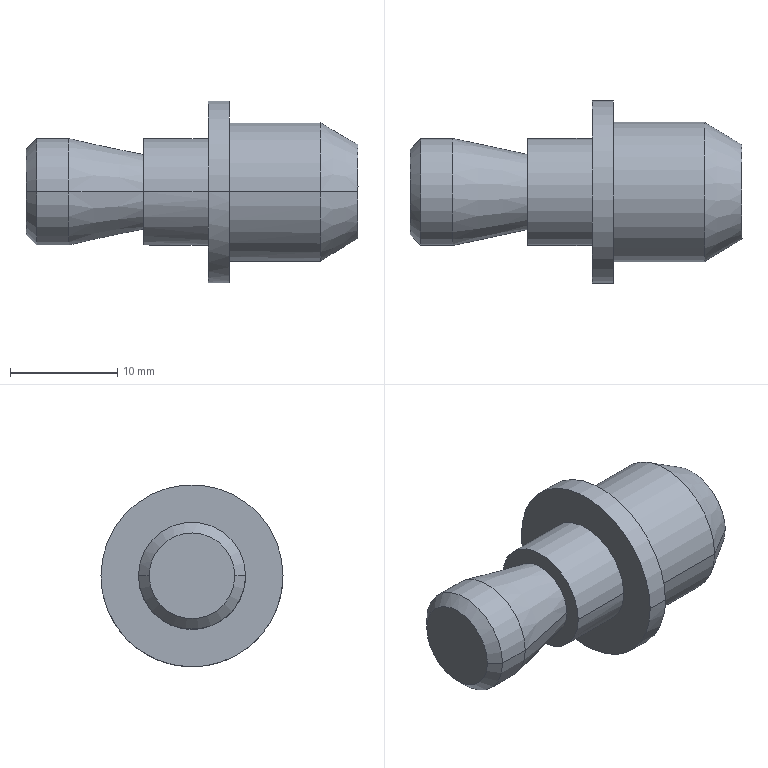Part | STEP file | Positioning_id2110_x_t | 1 solid | 19 faces | box 31 x 17 x 17 mm | volume 3085 mm3 | cylinder 8 | cone 6 | plane 5 | commonest cylinder face diameters 10 x4 13 x2 17 x2
STEP:
#1=CARTESIAN_POINT('',(0.,0.,0.));
#2=DIRECTION('',(0.,0.,1.));
#3=DIRECTION('',(1.,0.,0.));
#4=AXIS2_PLACEMENT_3D('',#1,#2,#3);
#5=CARTESIAN_POINT('',(-751.253,-22.5,364.));
#6=VERTEX_POINT('',#5);
#7=CARTESIAN_POINT('',(-747.753,-24.6,364.));
#8=VERTEX_POINT('',#7);
#9=CARTESIAN_POINT('',(-747.753,-24.6,364.));
#10=DIRECTION('',(0.8575,-0.5145,0.));
#11=VECTOR('',#10,1.);
#12=LINE('',#9,#11);
#13=CARTESIAN_POINT('',(-753.753,-29.,364.));
#14=DIRECTION('',(-1.,0.,0.));
#15=DIRECTION('',(0.,1.,0.));
#16=AXIS2_PLACEMENT_3D('',#13,#14,#15);
#17=CONICAL_SURFACE('',#16,8.,0.5404);
#18=CARTESIAN_POINT('',(0.,-6.));
#19=DIRECTION('',(0.,-1.));
#20=VECTOR('',#19,1.);
#21=LINE('',#18,#20);
#22=(GEOMETRIC_REPRESENTATION_CONTEXT(2)PARAMETRIC_REPRESENTATION_CONTEXT()REPRESENTATION_CONTEXT('',''));
#23=DEFINITIONAL_REPRESENTATION('',(#21),#22);
#24=PCURVE('',#17,#23);
#25=CARTESIAN_POINT('',(-753.753,-29.,364.));
#26=DIRECTION('',(-1.,0.,0.));
#27=DIRECTION('',(0.,1.,0.));
#28=AXIS2_PLACEMENT_3D('',#25,#26,#27);
#29=CONICAL_SURFACE('',#28,8.,0.5404);
#30=CARTESIAN_POINT('',(6.283,-6.));
#31=DIRECTION('',(0.,-1.));
#32=VECTOR('',#31,1.);
#33=LINE('',#30,#32);
#34=(GEOMETRIC_REPRESENTATION_CONTEXT(2)PARAMETRIC_REPRESENTATION_CONTEXT()REPRESENTATION_CONTEXT('',''));
#35=DEFINITIONAL_REPRESENTATION('',(#33),#34);
#36=PCURVE('',#29,#35);
#37=SURFACE_CURVE('',#12,(#24,#36),.PCURVE_S1.);
#38=EDGE_CURVE('',#6,#8,#37,.T.);
#39=ORIENTED_EDGE('',*,*,#38,.T.);
#40=CARTESIAN_POINT('',(-747.753,-33.4,364.));
#41=VERTEX_POINT('',#40);
#42=CARTESIAN_POINT('',(-747.753,-29.,364.));
#43=DIRECTION('',(1.,0.,0.));
#44=DIRECTION('',(0.,-1.,0.));
#45=AXIS2_PLACEMENT_3D('',#42,#43,#44);
#46=CIRCLE('',#45,4.4);
#47=CARTESIAN_POINT('',(3.142,-6.));
#48=DIRECTION('',(-1.,0.));
#49=VECTOR('',#48,1.);
#50=LINE('',#47,#49);
#51=(GEOMETRIC_REPRESENTATION_CONTEXT(2)PARAMETRIC_REPRESENTATION_CONTEXT()REPRESENTATION_CONTEXT('',''));
#52=DEFINITIONAL_REPRESENTATION('',(#50),#51);
#53=PCURVE('',#17,#52);
#54=CARTESIAN_POINT('',(-747.753,-29.,364.));
#55=DIRECTION('',(1.,0.,0.));
#56=DIRECTION('',(0.,1.,0.));
#57=AXIS2_PLACEMENT_3D('',#54,#55,#56);
#58=PLANE('',#57);
#59=CARTESIAN_POINT('',(0.,0.));
#60=DIRECTION('',(-1.,0.));
#61=AXIS2_PLACEMENT_2D('',#59,#60);
#62=CIRCLE('',#61,4.4);
#63=(GEOMETRIC_REPRESENTATION_CONTEXT(2)PARAMETRIC_REPRESENTATION_CONTEXT()REPRESENTATION_CONTEXT('',''));
#64=DEFINITIONAL_REPRESENTATION('',(#62),#63);
#65=PCURVE('',#58,#64);
#66=SURFACE_CURVE('',#46,(#53,#65),.PCURVE_S1.);
#67=EDGE_CURVE('',#41,#8,#66,.T.);
#68=ORIENTED_EDGE('',*,*,#67,.F.);
#69=CARTESIAN_POINT('',(-751.253,-35.5,364.));
#70=VERTEX_POINT('',#69);
#71=CARTESIAN_POINT('',(-747.753,-33.4,364.));
#72=DIRECTION('',(-0.8575,-0.5145,0.));
#73=VECTOR('',#72,1.);
#74=LINE('',#71,#73);
#75=CARTESIAN_POINT('',(3.142,-6.));
#76=DIRECTION('',(0.,1.));
#77=VECTOR('',#76,1.);
#78=LINE('',#75,#77);
#79=(GEOMETRIC_REPRESENTATION_CONTEXT(2)PARAMETRIC_REPRESENTATION_CONTEXT()REPRESENTATION_CONTEXT('',''));
#80=DEFINITIONAL_REPRESENTATION('',(#78),#79);
#81=PCURVE('',#17,#80);
#82=CARTESIAN_POINT('',(3.142,-6.));
#83=DIRECTION('',(0.,1.));
#84=VECTOR('',#83,1.);
#85=LINE('',#82,#84);
#86=(GEOMETRIC_REPRESENTATION_CONTEXT(2)PARAMETRIC_REPRESENTATION_CONTEXT()REPRESENTATION_CONTEXT('',''));
#87=DEFINITIONAL_REPRESENTATION('',(#85),#86);
#88=PCURVE('',#29,#87);
#89=SURFACE_CURVE('',#74,(#81,#88),.PCURVE_S1.);
#90=EDGE_CURVE('',#41,#70,#89,.T.);
#91=ORIENTED_EDGE('',*,*,#90,.T.);
#92=CARTESIAN_POINT('',(-751.253,-29.,364.));
#93=DIRECTION('',(-1.,0.,0.));
#94=DIRECTION('',(0.,1.,0.));
#95=AXIS2_PLACEMENT_3D('',#92,#93,#94);
#96=CIRCLE('',#95,6.5);
#97=CARTESIAN_POINT('',(0.,-2.5));
#98=DIRECTION('',(1.,0.));
#99=VECTOR('',#98,1.);
#100=LINE('',#97,#99);
#101=(GEOMETRIC_REPRESENTATION_CONTEXT(2)PARAMETRIC_REPRESENTATION_CONTEXT()REPRESENTATION_CONTEXT('',''));
#102=DEFINITIONAL_REPRESENTATION('',(#100),#101);
#103=PCURVE('',#17,#102);
#104=CARTESIAN_POINT('',(-758.753,-29.,364.));
#105=DIRECTION('',(-1.,0.,0.));
#106=DIRECTION('',(0.,1.,0.));
#107=AXIS2_PLACEMENT_3D('',#104,#105,#106);
#108=CYLINDRICAL_SURFACE('',#107,6.5);
#109=CARTESIAN_POINT('',(0.,-7.5));
#110=DIRECTION('',(1.,0.));
#111=VECTOR('',#110,1.);
#112=LINE('',#109,#111);
#113=(GEOMETRIC_REPRESENTATION_CONTEXT(2)PARAMETRIC_REPRESENTATION_CONTEXT()REPRESENTATION_CONTEXT('',''));
#114=DEFINITIONAL_REPRESENTATION('',(#112),#113);
#115=PCURVE('',#108,#114);
#116=SURFACE_CURVE('',#96,(#103,#115),.PCURVE_S1.);
#117=EDGE_CURVE('',#6,#70,#116,.T.);
#118=ORIENTED_EDGE('',*,*,#117,.F.);
#119=EDGE_LOOP('',(#39,#68,#91,#118));
#120=FACE_BOUND('',#119,.T.);
#121=ADVANCED_FACE('',(#120),#17,.T.);
#122=CARTESIAN_POINT('',(-759.753,-22.5,364.));
#123=VERTEX_POINT('',#122);
#124=CARTESIAN_POINT('',(-759.753,-22.5,364.));
#125=DIRECTION('',(-1.,0.,0.));
#126=VECTOR('',#125,1.);
#127=LINE('',#124,#126);
#128=CARTESIAN_POINT('',(-758.753,-29.,364.));
#129=DIRECTION('',(-1.,0.,0.));
#130=DIRECTION('',(0.,1.,0.));
#131=AXIS2_PLACEMENT_3D('',#128,#129,#130);
#132=CYLINDRICAL_SURFACE('',#131,6.5);
#133=CARTESIAN_POINT('',(6.283,1.));
#134=DIRECTION('',(0.,1.));
#135=VECTOR('',#134,1.);
#136=LINE('',#133,#135);
#137=(GEOMETRIC_REPRESENTATION_CONTEXT(2)PARAMETRIC_REPRESENTATION_CONTEXT()REPRESENTATION_CONTEXT('',''));
#138=DEFINITIONAL_REPRESENTATION('',(#136),#137);
#139=PCURVE('',#132,#138);
#140=CARTESIAN_POINT('',(0.,1.));
#141=DIRECTION('',(0.,1.));
#142=VECTOR('',#141,1.);
#143=LINE('',#140,#142);
#144=(GEOMETRIC_REPRESENTATION_CONTEXT(2)PARAMETRIC_REPRESENTATION_CONTEXT()REPRESENTATION_CONTEXT('',''));
#145=DEFINITIONAL_REPRESENTATION('',(#143),#144);
#146=PCURVE('',#108,#145);
#147=SURFACE_CURVE('',#127,(#139,#146),.PCURVE_S1.);
#148=EDGE_CURVE('',#6,#123,#147,.T.);
#149=ORIENTED_EDGE('',*,*,#148,.T.);
#150=CARTESIAN_POINT('',(-759.753,-35.5,364.));
#151=VERTEX_POINT('',#150);
#152=CARTESIAN_POINT('',(-759.753,-29.,364.));
#153=DIRECTION('',(1.,0.,0.));
#154=DIRECTION('',(0.,-1.,0.));
#155=AXIS2_PLACEMENT_3D('',#152,#153,#154);
#156=CIRCLE('',#155,6.5);
#157=CARTESIAN_POINT('',(9.425,1.));
#158=DIRECTION('',(-1.,0.));
#159=VECTOR('',#158,1.);
#160=LINE('',#157,#159);
#161=(GEOMETRIC_REPRESENTATION_CONTEXT(2)PARAMETRIC_REPRESENTATION_CONTEXT()REPRESENTATION_CONTEXT('',''));
#162=DEFINITIONAL_REPRESENTATION('',(#160),#161);
#163=PCURVE('',#132,#162);
#164=CARTESIAN_POINT('',(-759.753,-29.,364.));
#165=DIRECTION('',(1.,0.,0.));
#166=DIRECTION('',(0.,1.,0.));
#167=AXIS2_PLACEMENT_3D('',#164,#165,#166);
#168=PLANE('',#167);
#169=CARTESIAN_POINT('',(0.,0.));
#170=DIRECTION('',(-1.,0.));
#171=AXIS2_PLACEMENT_2D('',#169,#170);
#172=CIRCLE('',#171,6.5);
#173=(GEOMETRIC_REPRESENTATION_CONTEXT(2)PARAMETRIC_REPRESENTATION_CONTEXT()REPRESENTATION_CONTEXT('',''));
#174=DEFINITIONAL_REPRESENTATION('',(#172),#173);
#175=PCURVE('',#168,#174);
#176=SURFACE_CURVE('',#156,(#163,#175),.PCURVE_S1.);
#177=EDGE_CURVE('',#123,#151,#176,.T.);
#178=ORIENTED_EDGE('',*,*,#177,.T.);
#179=CARTESIAN_POINT('',(-759.753,-35.5,364.));
#180=DIRECTION('',(1.,0.,0.));
#181=VECTOR('',#180,1.);
#182=LINE('',#179,#181);
#183=CARTESIAN_POINT('',(3.142,1.));
#184=DIRECTION('',(0.,-1.));
#185=VECTOR('',#184,1.);
#186=LINE('',#183,#185);
#187=(GEOMETRIC_REPRESENTATION_CONTEXT(2)PARAMETRIC_REPRESENTATION_CONTEXT()REPRESENTATION_CONTEXT('',''));
#188=DEFINITIONAL_REPRESENTATION('',(#186),#187);
#189=PCURVE('',#132,#188);
#190=CARTESIAN_POINT('',(3.142,1.));
#191=DIRECTION('',(0.,-1.));
#192=VECTOR('',#191,1.);
#193=LINE('',#190,#192);
#194=(GEOMETRIC_REPRESENTATION_CONTEXT(2)PARAMETRIC_REPRESENTATION_CONTEXT()REPRESENTATION_CONTEXT('',''));
#195=DEFINITIONAL_REPRESENTATION('',(#193),#194);
#196=PCURVE('',#108,#195);
#197=SURFACE_CURVE('',#182,(#189,#196),.PCURVE_S1.);
#198=EDGE_CURVE('',#151,#70,#197,.T.);
#199=ORIENTED_EDGE('',*,*,#198,.T.);
#200=CARTESIAN_POINT('',(-751.253,-29.,364.));
#201=DIRECTION('',(-1.,0.,0.));
#202=DIRECTION('',(0.,-1.,0.));
#203=AXIS2_PLACEMENT_3D('',#200,#201,#202);
#204=CIRCLE('',#203,6.5);
#205=CARTESIAN_POINT('',(3.142,-7.5));
#206=DIRECTION('',(1.,0.));
#207=VECTOR('',#206,1.);
#208=LINE('',#205,#207);
#209=(GEOMETRIC_REPRESENTATION_CONTEXT(2)PARAMETRIC_REPRESENTATION_CONTEXT()REPRESENTATION_CONTEXT('',''));
#210=DEFINITIONAL_REPRESENTATION('',(#208),#209);
#211=PCURVE('',#132,#210);
#212=CARTESIAN_POINT('',(3.142,-2.5));
#213=DIRECTION('',(1.,0.));
#214=VECTOR('',#213,1.);
#215=LINE('',#212,#214);
#216=(GEOMETRIC_REPRESENTATION_CONTEXT(2)PARAMETRIC_REPRESENTATION_CONTEXT()REPRESENTATION_CONTEXT('',''));
#217=DEFINITIONAL_REPRESENTATION('',(#215),#216);
#218=PCURVE('',#29,#217);
#219=SURFACE_CURVE('',#204,(#211,#218),.PCURVE_S1.);
#220=EDGE_CURVE('',#70,#6,#219,.T.);
#221=ORIENTED_EDGE('',*,*,#220,.T.);
#222=EDGE_LOOP('',(#149,#178,#199,#221));
#223=FACE_BOUND('',#222,.T.);
#224=ADVANCED_FACE('',(#223),#132,.T.);
#225=ORIENTED_EDGE('',*,*,#67,.T.);
#226=CARTESIAN_POINT('',(-747.753,-24.6,364.));
#227=CARTESIAN_POINT('',(-747.753,-24.6,368.4));
#228=CARTESIAN_POINT('',(-747.753,-29.,370.6));
#229=CARTESIAN_POINT('',(-747.753,-33.4,368.4));
#230=CARTESIAN_POINT('',(-747.753,-33.4,364.));
#231=(BOUNDED_CURVE()B_SPLINE_CURVE(4,(#226,#227,#228,#229,#230),.UNSPECIFIED.,.F.,.F.)B_SPLINE_CURVE_WITH_KNOTS((5,5),(0.,1.),.PIECEWISE_BEZIER_KNOTS.)CURVE()GEOMETRIC_REPRESENTATION_ITEM()RATIONAL_B_SPLINE_CURVE((1.,0.7071,0.6667,0.7071,1.))REPRESENTATION_ITEM(''));
#232=CARTESIAN_POINT('',(4.4,0.));
#233=CARTESIAN_POINT('',(4.4,4.4));
#234=CARTESIAN_POINT('',(0.,6.6));
#235=CARTESIAN_POINT('',(-4.4,4.4));
#236=CARTESIAN_POINT('',(-4.4,0.));
#237=(BOUNDED_CURVE()B_SPLINE_CURVE(4,(#232,#233,#234,#235,#236),.UNSPECIFIED.,.F.,.F.)B_SPLINE_CURVE_WITH_KNOTS((5,5),(0.,1.),.PIECEWISE_BEZIER_KNOTS.)CURVE()GEOMETRIC_REPRESENTATION_ITEM()RATIONAL_B_SPLINE_CURVE((1.,0.7071,0.6667,0.7071,1.))REPRESENTATION_ITEM(''));
#238=(GEOMETRIC_REPRESENTATION_CONTEXT(2)PARAMETRIC_REPRESENTATION_CONTEXT()REPRESENTATION_CONTEXT('',''));
#239=DEFINITIONAL_REPRESENTATION('',(#237),#238);
#240=PCURVE('',#58,#239);
#241=CARTESIAN_POINT('',(6.283,-6.));
#242=CARTESIAN_POINT('',(6.24,-6.));
#243=CARTESIAN_POINT('',(6.153,-6.));
#244=CARTESIAN_POINT('',(6.02,-6.));
#245=CARTESIAN_POINT('',(5.883,-6.));
#246=CARTESIAN_POINT('',(5.744,-6.));
#247=CARTESIAN_POINT('',(5.602,-6.));
#248=CARTESIAN_POINT('',(5.457,-6.));
#249=CARTESIAN_POINT('',(5.311,-6.));
#250=CARTESIAN_POINT('',(5.163,-6.));
#251=CARTESIAN_POINT('',(5.013,-6.));
#252=CARTESIAN_POINT('',(4.863,-6.));
#253=CARTESIAN_POINT('',(4.712,-6.));
#254=CARTESIAN_POINT('',(4.562,-6.));
#255=CARTESIAN_POINT('',(4.412,-6.));
#256=CARTESIAN_POINT('',(4.262,-6.));
#257=CARTESIAN_POINT('',(4.114,-6.));
#258=CARTESIAN_POINT('',(3.968,-6.));
#259=CARTESIAN_POINT('',(3.823,-6.));
#260=CARTESIAN_POINT('',(3.681,-6.));
#261=CARTESIAN_POINT('',(3.542,-6.));
#262=CARTESIAN_POINT('',(3.405,-6.));
#263=CARTESIAN_POINT('',(3.271,-6.));
#264=CARTESIAN_POINT('',(3.184,-6.));
#265=CARTESIAN_POINT('',(3.142,-6.));
#266=B_SPLINE_CURVE_WITH_KNOTS('',3,(#241,#242,#243,#244,#245,#246,#247,#248,#249,#250,#251,#252,#253,#254,#255,#256,#257,#258,#259,#260,#261,#262,#263,#264,#265),.UNSPECIFIED.,.F.,.F.,(4,1,1,1,1,1,1,1,1,1,1,1,1,1,1,1,1,1,1,1,1,1,4),(0.,0.04545,0.09091,0.1364,0.1818,0.2273,0.2727,0.3182,0.3636,0.4091,0.4545,0.5,0.5455,0.5909,0.6364,0.6818,0.7273,0.7727,0.8182,0.8636,0.9091,0.9545,1.),.QUASI_UNIFORM_KNOTS.);
#267=(GEOMETRIC_REPRESENTATION_CONTEXT(2)PARAMETRIC_REPRESENTATION_CONTEXT()REPRESENTATION_CONTEXT('',''));
#268=DEFINITIONAL_REPRESENTATION('',(#266),#267);
#269=PCURVE('',#29,#268);
#270=SURFACE_CURVE('',#231,(#240,#269),.PCURVE_S1.);
#271=EDGE_CURVE('',#8,#41,#270,.T.);
#272=ORIENTED_EDGE('',*,*,#271,.T.);
#273=EDGE_LOOP('',(#225,#272));
#274=FACE_BOUND('',#273,.T.);
#275=ADVANCED_FACE('',(#274),#58,.T.);
#276=CARTESIAN_POINT('',(-767.753,-32.5,364.));
#277=VERTEX_POINT('',#276);
#278=CARTESIAN_POINT('',(-767.753,-25.5,364.));
#279=VERTEX_POINT('',#278);
#280=CARTESIAN_POINT('',(-767.753,-29.,364.));
#281=DIRECTION('',(1.,0.,0.));
#282=DIRECTION('',(0.,-1.,0.));
#283=AXIS2_PLACEMENT_3D('',#280,#281,#282);
#284=CIRCLE('',#283,3.5);
#285=CARTESIAN_POINT('',(-767.753,-29.,364.));
#286=DIRECTION('',(1.,0.,0.));
#287=DIRECTION('',(0.,1.,0.));
#288=AXIS2_PLACEMENT_3D('',#285,#286,#287);
#289=PLANE('',#288);
#290=CARTESIAN_POINT('',(0.,0.));
#291=DIRECTION('',(-1.,0.));
#292=AXIS2_PLACEMENT_2D('',#290,#291);
#293=CIRCLE('',#292,3.5);
#294=(GEOMETRIC_REPRESENTATION_CONTEXT(2)PARAMETRIC_REPRESENTATION_CONTEXT()REPRESENTATION_CONTEXT('',''));
#295=DEFINITIONAL_REPRESENTATION('',(#293),#294);
#296=PCURVE('',#289,#295);
#297=CARTESIAN_POINT('',(-774.753,-29.,364.));
#298=DIRECTION('',(-1.,0.,0.));
#299=DIRECTION('',(0.,1.,0.));
#300=AXIS2_PLACEMENT_3D('',#297,#298,#299);
#301=CONICAL_SURFACE('',#300,5.,0.2111);
#302=CARTESIAN_POINT('',(3.142,-7.));
#303=DIRECTION('',(-1.,0.));
#304=VECTOR('',#303,1.);
#305=LINE('',#302,#304);
#306=(GEOMETRIC_REPRESENTATION_CONTEXT(2)PARAMETRIC_REPRESENTATION_CONTEXT()REPRESENTATION_CONTEXT('',''));
#307=DEFINITIONAL_REPRESENTATION('',(#305),#306);
#308=PCURVE('',#301,#307);
#309=SURFACE_CURVE('',#284,(#296,#308),.PCURVE_S1.);
#310=EDGE_CURVE('',#277,#279,#309,.T.);
#311=ORIENTED_EDGE('',*,*,#310,.T.);
#312=CARTESIAN_POINT('',(-767.753,-29.,364.));
#313=DIRECTION('',(1.,0.,0.));
#314=DIRECTION('',(0.,1.,0.));
#315=AXIS2_PLACEMENT_3D('',#312,#313,#314);
#316=CIRCLE('',#315,3.5);
#317=CARTESIAN_POINT('',(0.,0.));
#318=DIRECTION('',(1.,0.));
#319=AXIS2_PLACEMENT_2D('',#317,#318);
#320=CIRCLE('',#319,3.5);
#321=(GEOMETRIC_REPRESENTATION_CONTEXT(2)PARAMETRIC_REPRESENTATION_CONTEXT()REPRESENTATION_CONTEXT('',''));
#322=DEFINITIONAL_REPRESENTATION('',(#320),#321);
#323=PCURVE('',#289,#322);
#324=CARTESIAN_POINT('',(-774.753,-29.,364.));
#325=DIRECTION('',(-1.,0.,0.));
#326=DIRECTION('',(0.,1.,0.));
#327=AXIS2_PLACEMENT_3D('',#324,#325,#326);
#328=CONICAL_SURFACE('',#327,5.,0.2111);
#329=CARTESIAN_POINT('',(6.283,-7.));
#330=DIRECTION('',(-1.,0.));
#331=VECTOR('',#330,1.);
#332=LINE('',#329,#331);
#333=(GEOMETRIC_REPRESENTATION_CONTEXT(2)PARAMETRIC_REPRESENTATION_CONTEXT()REPRESENTATION_CONTEXT('',''));
#334=DEFINITIONAL_REPRESENTATION('',(#332),#333);
#335=PCURVE('',#328,#334);
#336=SURFACE_CURVE('',#316,(#323,#335),.PCURVE_S1.);
#337=EDGE_CURVE('',#279,#277,#336,.T.);
#338=ORIENTED_EDGE('',*,*,#337,.T.);
#339=EDGE_LOOP('',(#311,#338));
#340=FACE_BOUND('',#339,.T.);
#341=CARTESIAN_POINT('',(-767.753,-34.,364.));
#342=VERTEX_POINT('',#341);
#343=CARTESIAN_POINT('',(-767.753,-24.,364.));
#344=VERTEX_POINT('',#343);
#345=CARTESIAN_POINT('',(-767.753,-29.,364.));
#346=DIRECTION('',(-1.,0.,0.));
#347=DIRECTION('',(0.,-1.,0.));
#348=AXIS2_PLACEMENT_3D('',#345,#346,#347);
#349=CIRCLE('',#348,5.);
#350=CARTESIAN_POINT('',(-5.,0.));
#351=CARTESIAN_POINT('',(-5.,8.66));
#352=CARTESIAN_POINT('',(2.5,4.33));
#353=CARTESIAN_POINT('',(10.,0.));
#354=CARTESIAN_POINT('',(2.5,-4.33));
#355=CARTESIAN_POINT('',(-5.,-8.66));
#356=CARTESIAN_POINT('',(-5.,0.));
#357=(BOUNDED_CURVE()B_SPLINE_CURVE(2,(#350,#351,#352,#353,#354,#355,#356),.UNSPECIFIED.,.T.,.F.)B_SPLINE_CURVE_WITH_KNOTS((1,2,2,2,2,1),(-2.094,0.,2.094,4.189,6.283,8.378),.UNSPECIFIED.)CURVE()GEOMETRIC_REPRESENTATION_ITEM()RATIONAL_B_SPLINE_CURVE((1.,0.5,1.,0.5,1.,0.5,1.))REPRESENTATION_ITEM(''));
#358=(GEOMETRIC_REPRESENTATION_CONTEXT(2)PARAMETRIC_REPRESENTATION_CONTEXT()REPRESENTATION_CONTEXT('',''));
#359=DEFINITIONAL_REPRESENTATION('',(#357),#358);
#360=PCURVE('',#289,#359);
#361=CARTESIAN_POINT('',(-768.753,-29.,364.));
#362=DIRECTION('',(-1.,0.,0.));
#363=DIRECTION('',(0.,1.,0.));
#364=AXIS2_PLACEMENT_3D('',#361,#362,#363);
#365=CYLINDRICAL_SURFACE('',#364,5.);
#366=CARTESIAN_POINT('',(3.142,-1.));
#367=DIRECTION('',(1.,0.));
#368=VECTOR('',#367,1.);
#369=LINE('',#366,#368);
#370=(GEOMETRIC_REPRESENTATION_CONTEXT(2)PARAMETRIC_REPRESENTATION_CONTEXT()REPRESENTATION_CONTEXT('',''));
#371=DEFINITIONAL_REPRESENTATION('',(#369),#370);
#372=PCURVE('',#365,#371);
#373=SURFACE_CURVE('',#349,(#360,#372),.PCURVE_S1.);
#374=EDGE_CURVE('',#342,#344,#373,.T.);
#375=ORIENTED_EDGE('',*,*,#374,.T.);
#376=CARTESIAN_POINT('',(-767.753,-29.,364.));
#377=DIRECTION('',(-1.,0.,0.));
#378=DIRECTION('',(0.,1.,0.));
#379=AXIS2_PLACEMENT_3D('',#376,#377,#378);
#380=CIRCLE('',#379,5.);
#381=CARTESIAN_POINT('',(5.,0.));
#382=CARTESIAN_POINT('',(5.,-8.66));
#383=CARTESIAN_POINT('',(-2.5,-4.33));
#384=CARTESIAN_POINT('',(-10.,0.));
#385=CARTESIAN_POINT('',(-2.5,4.33));
#386=CARTESIAN_POINT('',(5.,8.66));
#387=CARTESIAN_POINT('',(5.,0.));
#388=(BOUNDED_CURVE()B_SPLINE_CURVE(2,(#381,#382,#383,#384,#385,#386,#387),.UNSPECIFIED.,.T.,.F.)B_SPLINE_CURVE_WITH_KNOTS((1,2,2,2,2,1),(-2.094,0.,2.094,4.189,6.283,8.378),.UNSPECIFIED.)CURVE()GEOMETRIC_REPRESENTATION_ITEM()RATIONAL_B_SPLINE_CURVE((1.,0.5,1.,0.5,1.,0.5,1.))REPRESENTATION_ITEM(''));
#389=(GEOMETRIC_REPRESENTATION_CONTEXT(2)PARAMETRIC_REPRESENTATION_CONTEXT()REPRESENTATION_CONTEXT('',''));
#390=DEFINITIONAL_REPRESENTATION('',(#388),#389);
#391=PCURVE('',#289,#390);
#392=CARTESIAN_POINT('',(-768.753,-29.,364.));
#393=DIRECTION('',(-1.,0.,0.));
#394=DIRECTION('',(0.,1.,0.));
#395=AXIS2_PLACEMENT_3D('',#392,#393,#394);
#396=CYLINDRICAL_SURFACE('',#395,5.);
#397=CARTESIAN_POINT('',(0.,-1.));
#398=DIRECTION('',(1.,0.));
#399=VECTOR('',#398,1.);
#400=LINE('',#397,#399);
#401=(GEOMETRIC_REPRESENTATION_CONTEXT(2)PARAMETRIC_REPRESENTATION_CONTEXT()REPRESENTATION_CONTEXT('',''));
#402=DEFINITIONAL_REPRESENTATION('',(#400),#401);
#403=PCURVE('',#396,#402);
#404=SURFACE_CURVE('',#380,(#391,#403),.PCURVE_S1.);
#405=EDGE_CURVE('',#344,#342,#404,.T.);
#406=ORIENTED_EDGE('',*,*,#405,.T.);
#407=EDGE_LOOP('',(#375,#406));
#408=FACE_BOUND('',#407,.T.);
#409=ADVANCED_FACE('',(#340,#408),#289,.F.);
#410=CARTESIAN_POINT('',(-761.753,-24.,364.));
#411=VERTEX_POINT('',#410);
#412=CARTESIAN_POINT('',(-767.753,-24.,364.));
#413=DIRECTION('',(-1.,0.,0.));
#414=VECTOR('',#413,1.);
#415=LINE('',#412,#414);
#416=CARTESIAN_POINT('',(6.283,-1.));
#417=DIRECTION('',(0.,1.));
#418=VECTOR('',#417,1.);
#419=LINE('',#416,#418);
#420=(GEOMETRIC_REPRESENTATION_CONTEXT(2)PARAMETRIC_REPRESENTATION_CONTEXT()REPRESENTATION_CONTEXT('',''));
#421=DEFINITIONAL_REPRESENTATION('',(#419),#420);
#422=PCURVE('',#365,#421);
#423=CARTESIAN_POINT('',(0.,-1.));
#424=DIRECTION('',(0.,1.));
#425=VECTOR('',#424,1.);
#426=LINE('',#423,#425);
#427=(GEOMETRIC_REPRESENTATION_CONTEXT(2)PARAMETRIC_REPRESENTATION_CONTEXT()REPRESENTATION_CONTEXT('',''));
#428=DEFINITIONAL_REPRESENTATION('',(#426),#427);
#429=PCURVE('',#396,#428);
#430=SURFACE_CURVE('',#415,(#422,#429),.PCURVE_S1.);
#431=EDGE_CURVE('',#411,#344,#430,.T.);
#432=ORIENTED_EDGE('',*,*,#431,.T.);
#433=ORIENTED_EDGE('',*,*,#374,.F.);
#434=CARTESIAN_POINT('',(-761.753,-34.,364.));
#435=VERTEX_POINT('',#434);
#436=CARTESIAN_POINT('',(-767.753,-34.,364.));
#437=DIRECTION('',(1.,0.,0.));
#438=VECTOR('',#437,1.);
#439=LINE('',#436,#438);
#440=CARTESIAN_POINT('',(3.142,-1.));
#441=DIRECTION('',(0.,-1.));
#442=VECTOR('',#441,1.);
#443=LINE('',#440,#442);
#444=(GEOMETRIC_REPRESENTATION_CONTEXT(2)PARAMETRIC_REPRESENTATION_CONTEXT()REPRESENTATION_CONTEXT('',''));
#445=DEFINITIONAL_REPRESENTATION('',(#443),#444);
#446=PCURVE('',#365,#445);
#447=CARTESIAN_POINT('',(3.142,-1.));
#448=DIRECTION('',(0.,-1.));
#449=VECTOR('',#448,1.);
#450=LINE('',#447,#449);
#451=(GEOMETRIC_REPRESENTATION_CONTEXT(2)PARAMETRIC_REPRESENTATION_CONTEXT()REPRESENTATION_CONTEXT('',''));
#452=DEFINITIONAL_REPRESENTATION('',(#450),#451);
#453=PCURVE('',#396,#452);
#454=SURFACE_CURVE('',#439,(#446,#453),.PCURVE_S1.);
#455=EDGE_CURVE('',#342,#435,#454,.T.);
#456=ORIENTED_EDGE('',*,*,#455,.T.);
#457=CARTESIAN_POINT('',(-761.753,-29.,364.));
#458=DIRECTION('',(-1.,0.,0.));
#459=DIRECTION('',(0.,-1.,0.));
#460=AXIS2_PLACEMENT_3D('',#457,#458,#459);
#461=CIRCLE('',#460,5.);
#462=CARTESIAN_POINT('',(3.142,-7.));
#463=DIRECTION('',(1.,0.));
#464=VECTOR('',#463,1.);
#465=LINE('',#462,#464);
#466=(GEOMETRIC_REPRESENTATION_CONTEXT(2)PARAMETRIC_REPRESENTATION_CONTEXT()REPRESENTATION_CONTEXT('',''));
#467=DEFINITIONAL_REPRESENTATION('',(#465),#466);
#468=PCURVE('',#365,#467);
#469=CARTESIAN_POINT('',(-761.753,-29.,364.));
#470=DIRECTION('',(-1.,0.,0.));
#471=DIRECTION('',(0.,-1.,0.));
#472=AXIS2_PLACEMENT_3D('',#469,#470,#471);
#473=PLANE('',#472);
#474=CARTESIAN_POINT('',(0.,0.));
#475=DIRECTION('',(1.,0.));
#476=AXIS2_PLACEMENT_2D('',#474,#475);
#477=CIRCLE('',#476,5.);
#478=(GEOMETRIC_REPRESENTATION_CONTEXT(2)PARAMETRIC_REPRESENTATION_CONTEXT()REPRESENTATION_CONTEXT('',''));
#479=DEFINITIONAL_REPRESENTATION('',(#477),#478);
#480=PCURVE('',#473,#479);
#481=SURFACE_CURVE('',#461,(#468,#480),.PCURVE_S1.);
#482=EDGE_CURVE('',#435,#411,#481,.T.);
#483=ORIENTED_EDGE('',*,*,#482,.T.);
#484=EDGE_LOOP('',(#432,#433,#456,#483));
#485=FACE_BOUND('',#484,.T.);
#486=ADVANCED_FACE('',(#485),#365,.T.);
#487=CARTESIAN_POINT('',(-774.753,-24.,364.));
#488=VERTEX_POINT('',#487);
#489=CARTESIAN_POINT('',(-767.753,-25.5,364.));
#490=DIRECTION('',(0.9778,-0.2095,0.));
#491=VECTOR('',#490,1.);
#492=LINE('',#489,#491);
#493=CARTESIAN_POINT('',(0.,-7.));
#494=DIRECTION('',(0.,-1.));
#495=VECTOR('',#494,1.);
#496=LINE('',#493,#495);
#497=(GEOMETRIC_REPRESENTATION_CONTEXT(2)PARAMETRIC_REPRESENTATION_CONTEXT()REPRESENTATION_CONTEXT('',''));
#498=DEFINITIONAL_REPRESENTATION('',(#496),#497);
#499=PCURVE('',#301,#498);
#500=CARTESIAN_POINT('',(6.283,-7.));
#501=DIRECTION('',(0.,-1.));
#502=VECTOR('',#501,1.);
#503=LINE('',#500,#502);
#504=(GEOMETRIC_REPRESENTATION_CONTEXT(2)PARAMETRIC_REPRESENTATION_CONTEXT()REPRESENTATION_CONTEXT('',''));
#505=DEFINITIONAL_REPRESENTATION('',(#503),#504);
#506=PCURVE('',#328,#505);
#507=SURFACE_CURVE('',#492,(#499,#506),.PCURVE_S1.);
#508=EDGE_CURVE('',#488,#279,#507,.T.);
#509=ORIENTED_EDGE('',*,*,#508,.T.);
#510=ORIENTED_EDGE('',*,*,#310,.F.);
#511=CARTESIAN_POINT('',(-774.753,-34.,364.));
#512=VERTEX_POINT('',#511);
#513=CARTESIAN_POINT('',(-767.753,-32.5,364.));
#514=DIRECTION('',(-0.9778,-0.2095,0.));
#515=VECTOR('',#514,1.);
#516=LINE('',#513,#515);
#517=CARTESIAN_POINT('',(3.142,-7.));
#518=DIRECTION('',(0.,1.));
#519=VECTOR('',#518,1.);
#520=LINE('',#517,#519);
#521=(GEOMETRIC_REPRESENTATION_CONTEXT(2)PARAMETRIC_REPRESENTATION_CONTEXT()REPRESENTATION_CONTEXT('',''));
#522=DEFINITIONAL_REPRESENTATION('',(#520),#521);
#523=PCURVE('',#301,#522);
#524=CARTESIAN_POINT('',(3.142,-7.));
#525=DIRECTION('',(0.,1.));
#526=VECTOR('',#525,1.);
#527=LINE('',#524,#526);
#528=(GEOMETRIC_REPRESENTATION_CONTEXT(2)PARAMETRIC_REPRESENTATION_CONTEXT()REPRESENTATION_CONTEXT('',''));
#529=DEFINITIONAL_REPRESENTATION('',(#527),#528);
#530=PCURVE('',#328,#529);
#531=SURFACE_CURVE('',#516,(#523,#530),.PCURVE_S1.);
#532=EDGE_CURVE('',#277,#512,#531,.T.);
#533=ORIENTED_EDGE('',*,*,#532,.T.);
#534=CARTESIAN_POINT('',(-774.753,-29.,364.));
#535=DIRECTION('',(-1.,0.,0.));
#536=DIRECTION('',(0.,1.,0.));
#537=AXIS2_PLACEMENT_3D('',#534,#535,#536);
#538=CIRCLE('',#537,5.);
#539=CARTESIAN_POINT('',(0.,0.));
#540=DIRECTION('',(1.,0.));
#541=VECTOR('',#540,1.);
#542=LINE('',#539,#541);
#543=(GEOMETRIC_REPRESENTATION_CONTEXT(2)PARAMETRIC_REPRESENTATION_CONTEXT()REPRESENTATION_CONTEXT('',''));
#544=DEFINITIONAL_REPRESENTATION('',(#542),#543);
#545=PCURVE('',#301,#544);
#546=CARTESIAN_POINT('',(-768.753,-29.,364.));
#547=DIRECTION('',(-1.,0.,0.));
#548=DIRECTION('',(0.,1.,0.));
#549=AXIS2_PLACEMENT_3D('',#546,#547,#548);
#550=CYLINDRICAL_SURFACE('',#549,5.);
#551=CARTESIAN_POINT('',(0.,6.));
#552=DIRECTION('',(1.,0.));
#553=VECTOR('',#552,1.);
#554=LINE('',#551,#553);
#555=(GEOMETRIC_REPRESENTATION_CONTEXT(2)PARAMETRIC_REPRESENTATION_CONTEXT()REPRESENTATION_CONTEXT('',''));
#556=DEFINITIONAL_REPRESENTATION('',(#554),#555);
#557=PCURVE('',#550,#556);
#558=SURFACE_CURVE('',#538,(#545,#557),.PCURVE_S1.);
#559=EDGE_CURVE('',#488,#512,#558,.T.);
#560=ORIENTED_EDGE('',*,*,#559,.F.);
#561=EDGE_LOOP('',(#509,#510,#533,#560));
#562=FACE_BOUND('',#561,.T.);
#563=ADVANCED_FACE('',(#562),#301,.T.);
#564=CARTESIAN_POINT('',(-777.753,-34.,364.));
#565=VERTEX_POINT('',#564);
#566=CARTESIAN_POINT('',(-778.753,-33.,364.));
#567=VERTEX_POINT('',#566);
#568=CARTESIAN_POINT('',(-778.753,-33.,364.));
#569=DIRECTION('',(-0.7071,0.7071,0.));
#570=VECTOR('',#569,1.);
#571=LINE('',#568,#570);
#572=CARTESIAN_POINT('',(-777.753,-29.,364.));
#573=DIRECTION('',(1.,0.,0.));
#574=DIRECTION('',(0.,-1.,0.));
#575=AXIS2_PLACEMENT_3D('',#572,#573,#574);
#576=CONICAL_SURFACE('',#575,5.,0.7854);
#577=CARTESIAN_POINT('',(0.,-1.));
#578=DIRECTION('',(0.,-1.));
#579=VECTOR('',#578,1.);
#580=LINE('',#577,#579);
#581=(GEOMETRIC_REPRESENTATION_CONTEXT(2)PARAMETRIC_REPRESENTATION_CONTEXT()REPRESENTATION_CONTEXT('',''));
#582=DEFINITIONAL_REPRESENTATION('',(#580),#581);
#583=PCURVE('',#576,#582);
#584=CARTESIAN_POINT('',(-777.753,-29.,364.));
#585=DIRECTION('',(1.,0.,0.));
#586=DIRECTION('',(0.,-1.,0.));
#587=AXIS2_PLACEMENT_3D('',#584,#585,#586);
#588=CONICAL_SURFACE('',#587,5.,0.7854);
#589=CARTESIAN_POINT('',(6.283,-1.));
#590=DIRECTION('',(0.,-1.));
#591=VECTOR('',#590,1.);
#592=LINE('',#589,#591);
#593=(GEOMETRIC_REPRESENTATION_CONTEXT(2)PARAMETRIC_REPRESENTATION_CONTEXT()REPRESENTATION_CONTEXT('',''));
#594=DEFINITIONAL_REPRESENTATION('',(#592),#593);
#595=PCURVE('',#588,#594);
#596=SURFACE_CURVE('',#571,(#583,#595),.PCURVE_S1.);
#597=EDGE_CURVE('',#565,#567,#596,.T.);
#598=ORIENTED_EDGE('',*,*,#597,.T.);
#599=CARTESIAN_POINT('',(-778.753,-25.,364.));
#600=VERTEX_POINT('',#599);
#601=CARTESIAN_POINT('',(-778.753,-29.,364.));
#602=DIRECTION('',(-1.,0.,0.));
#603=DIRECTION('',(0.,1.,0.));
#604=AXIS2_PLACEMENT_3D('',#601,#602,#603);
#605=CIRCLE('',#604,4.);
#606=CARTESIAN_POINT('',(3.142,-1.));
#607=DIRECTION('',(-1.,0.));
#608=VECTOR('',#607,1.);
#609=LINE('',#606,#608);
#610=(GEOMETRIC_REPRESENTATION_CONTEXT(2)PARAMETRIC_REPRESENTATION_CONTEXT()REPRESENTATION_CONTEXT('',''));
#611=DEFINITIONAL_REPRESENTATION('',(#609),#610);
#612=PCURVE('',#576,#611);
#613=CARTESIAN_POINT('',(-778.753,-29.,364.));
#614=DIRECTION('',(-1.,0.,0.));
#615=DIRECTION('',(0.,-1.,0.));
#616=AXIS2_PLACEMENT_3D('',#613,#614,#615);
#617=PLANE('',#616);
#618=CARTESIAN_POINT('',(0.,0.));
#619=DIRECTION('',(-1.,0.));
#620=AXIS2_PLACEMENT_2D('',#618,#619);
#621=CIRCLE('',#620,4.);
#622=(GEOMETRIC_REPRESENTATION_CONTEXT(2)PARAMETRIC_REPRESENTATION_CONTEXT()REPRESENTATION_CONTEXT('',''));
#623=DEFINITIONAL_REPRESENTATION('',(#621),#622);
#624=PCURVE('',#617,#623);
#625=SURFACE_CURVE('',#605,(#612,#624),.PCURVE_S1.);
#626=EDGE_CURVE('',#600,#567,#625,.T.);
#627=ORIENTED_EDGE('',*,*,#626,.F.);
#628=CARTESIAN_POINT('',(-777.753,-24.,364.));
#629=VERTEX_POINT('',#628);
#630=CARTESIAN_POINT('',(-778.753,-25.,364.));
#631=DIRECTION('',(0.7071,0.7071,0.));
#632=VECTOR('',#631,1.);
#633=LINE('',#630,#632);
#634=CARTESIAN_POINT('',(3.142,-1.));
#635=DIRECTION('',(0.,1.));
#636=VECTOR('',#635,1.);
#637=LINE('',#634,#636);
#638=(GEOMETRIC_REPRESENTATION_CONTEXT(2)PARAMETRIC_REPRESENTATION_CONTEXT()REPRESENTATION_CONTEXT('',''));
#639=DEFINITIONAL_REPRESENTATION('',(#637),#638);
#640=PCURVE('',#576,#639);
#641=CARTESIAN_POINT('',(3.142,-1.));
#642=DIRECTION('',(0.,1.));
#643=VECTOR('',#642,1.);
#644=LINE('',#641,#643);
#645=(GEOMETRIC_REPRESENTATION_CONTEXT(2)PARAMETRIC_REPRESENTATION_CONTEXT()REPRESENTATION_CONTEXT('',''));
#646=DEFINITIONAL_REPRESENTATION('',(#644),#645);
#647=PCURVE('',#588,#646);
#648=SURFACE_CURVE('',#633,(#640,#647),.PCURVE_S1.);
#649=EDGE_CURVE('',#600,#629,#648,.T.);
#650=ORIENTED_EDGE('',*,*,#649,.T.);
#651=CARTESIAN_POINT('',(-777.753,-29.,364.));
#652=DIRECTION('',(1.,0.,0.));
#653=DIRECTION('',(0.,-1.,0.));
#654=AXIS2_PLACEMENT_3D('',#651,#652,#653);
#655=CIRCLE('',#654,5.);
#656=CARTESIAN_POINT('',(0.,0.));
#657=DIRECTION('',(1.,0.));
#658=VECTOR('',#657,1.);
#659=LINE('',#656,#658);
#660=(GEOMETRIC_REPRESENTATION_CONTEXT(2)PARAMETRIC_REPRESENTATION_CONTEXT()REPRESENTATION_CONTEXT('',''));
#661=DEFINITIONAL_REPRESENTATION('',(#659),#660);
#662=PCURVE('',#576,#661);
#663=CARTESIAN_POINT('',(3.142,9.));
#664=DIRECTION('',(-1.,0.));
#665=VECTOR('',#664,1.);
#666=LINE('',#663,#665);
#667=(GEOMETRIC_REPRESENTATION_CONTEXT(2)PARAMETRIC_REPRESENTATION_CONTEXT()REPRESENTATION_CONTEXT('',''));
#668=DEFINITIONAL_REPRESENTATION('',(#666),#667);
#669=PCURVE('',#550,#668);
#670=SURFACE_CURVE('',#655,(#662,#669),.PCURVE_S1.);
#671=EDGE_CURVE('',#565,#629,#670,.T.);
#672=ORIENTED_EDGE('',*,*,#671,.F.);
#673=EDGE_LOOP('',(#598,#627,#650,#672));
#674=FACE_BOUND('',#673,.T.);
#675=ADVANCED_FACE('',(#674),#576,.T.);
#676=CARTESIAN_POINT('',(-777.753,-24.,364.));
#677=DIRECTION('',(1.,0.,0.));
#678=VECTOR('',#677,1.);
#679=LINE('',#676,#678);
#680=CARTESIAN_POINT('',(-768.753,-29.,364.));
#681=DIRECTION('',(-1.,0.,0.));
#682=DIRECTION('',(0.,1.,0.));
#683=AXIS2_PLACEMENT_3D('',#680,#681,#682);
#684=CYLINDRICAL_SURFACE('',#683,5.);
#685=CARTESIAN_POINT('',(6.283,9.));
#686=DIRECTION('',(0.,-1.));
#687=VECTOR('',#686,1.);
#688=LINE('',#685,#687);
#689=(GEOMETRIC_REPRESENTATION_CONTEXT(2)PARAMETRIC_REPRESENTATION_CONTEXT()REPRESENTATION_CONTEXT('',''));
#690=DEFINITIONAL_REPRESENTATION('',(#688),#689);
#691=PCURVE('',#684,#690);
#692=CARTESIAN_POINT('',(0.,9.));
#693=DIRECTION('',(0.,-1.));
#694=VECTOR('',#693,1.);
#695=LINE('',#692,#694);
#696=(GEOMETRIC_REPRESENTATION_CONTEXT(2)PARAMETRIC_REPRESENTATION_CONTEXT()REPRESENTATION_CONTEXT('',''));
#697=DEFINITIONAL_REPRESENTATION('',(#695),#696);
#698=PCURVE('',#550,#697);
#699=SURFACE_CURVE('',#679,(#691,#698),.PCURVE_S1.);
#700=EDGE_CURVE('',#629,#488,#699,.T.);
#701=ORIENTED_EDGE('',*,*,#700,.F.);
#702=CARTESIAN_POINT('',(-777.753,-29.,364.));
#703=DIRECTION('',(1.,0.,0.));
#704=DIRECTION('',(0.,1.,0.));
#705=AXIS2_PLACEMENT_3D('',#702,#703,#704);
#706=CIRCLE('',#705,5.);
#707=CARTESIAN_POINT('',(6.283,9.));
#708=DIRECTION('',(-1.,0.));
#709=VECTOR('',#708,1.);
#710=LINE('',#707,#709);
#711=(GEOMETRIC_REPRESENTATION_CONTEXT(2)PARAMETRIC_REPRESENTATION_CONTEXT()REPRESENTATION_CONTEXT('',''));
#712=DEFINITIONAL_REPRESENTATION('',(#710),#711);
#713=PCURVE('',#684,#712);
#714=CARTESIAN_POINT('',(3.142,0.));
#715=DIRECTION('',(1.,0.));
#716=VECTOR('',#715,1.);
#717=LINE('',#714,#716);
#718=(GEOMETRIC_REPRESENTATION_CONTEXT(2)PARAMETRIC_REPRESENTATION_CONTEXT()REPRESENTATION_CONTEXT('',''));
#719=DEFINITIONAL_REPRESENTATION('',(#717),#718);
#720=PCURVE('',#588,#719);
#721=SURFACE_CURVE('',#706,(#713,#720),.PCURVE_S1.);
#722=EDGE_CURVE('',#629,#565,#721,.T.);
#723=ORIENTED_EDGE('',*,*,#722,.T.);
#724=CARTESIAN_POINT('',(-777.753,-34.,364.));
#725=DIRECTION('',(-1.,0.,0.));
#726=VECTOR('',#725,1.);
#727=LINE('',#724,#726);
#728=CARTESIAN_POINT('',(3.142,9.));
#729=DIRECTION('',(0.,1.));
#730=VECTOR('',#729,1.);
#731=LINE('',#728,#730);
#732=(GEOMETRIC_REPRESENTATION_CONTEXT(2)PARAMETRIC_REPRESENTATION_CONTEXT()REPRESENTATION_CONTEXT('',''));
#733=DEFINITIONAL_REPRESENTATION('',(#731),#732);
#734=PCURVE('',#684,#733);
#735=CARTESIAN_POINT('',(3.142,9.));
#736=DIRECTION('',(0.,1.));
#737=VECTOR('',#736,1.);
#738=LINE('',#735,#737);
#739=(GEOMETRIC_REPRESENTATION_CONTEXT(2)PARAMETRIC_REPRESENTATION_CONTEXT()REPRESENTATION_CONTEXT('',''));
#740=DEFINITIONAL_REPRESENTATION('',(#738),#739);
#741=PCURVE('',#550,#740);
#742=SURFACE_CURVE('',#727,(#734,#741),.PCURVE_S1.);
#743=EDGE_CURVE('',#512,#565,#742,.T.);
#744=ORIENTED_EDGE('',*,*,#743,.F.);
#745=CARTESIAN_POINT('',(-774.753,-29.,364.));
#746=DIRECTION('',(-1.,0.,0.));
#747=DIRECTION('',(0.,-1.,0.));
#748=AXIS2_PLACEMENT_3D('',#745,#746,#747);
#749=CIRCLE('',#748,5.);
#750=CARTESIAN_POINT('',(3.142,6.));
#751=DIRECTION('',(1.,0.));
#752=VECTOR('',#751,1.);
#753=LINE('',#750,#752);
#754=(GEOMETRIC_REPRESENTATION_CONTEXT(2)PARAMETRIC_REPRESENTATION_CONTEXT()REPRESENTATION_CONTEXT('',''));
#755=DEFINITIONAL_REPRESENTATION('',(#753),#754);
#756=PCURVE('',#684,#755);
#757=CARTESIAN_POINT('',(3.142,0.));
#758=DIRECTION('',(1.,0.));
#759=VECTOR('',#758,1.);
#760=LINE('',#757,#759);
#761=(GEOMETRIC_REPRESENTATION_CONTEXT(2)PARAMETRIC_REPRESENTATION_CONTEXT()REPRESENTATION_CONTEXT('',''));
#762=DEFINITIONAL_REPRESENTATION('',(#760),#761);
#763=PCURVE('',#328,#762);
#764=SURFACE_CURVE('',#749,(#756,#763),.PCURVE_S1.);
#765=EDGE_CURVE('',#512,#488,#764,.T.);
#766=ORIENTED_EDGE('',*,*,#765,.T.);
#767=EDGE_LOOP('',(#701,#723,#744,#766));
#768=FACE_BOUND('',#767,.T.);
#769=ADVANCED_FACE('',(#768),#684,.T.);
#770=ORIENTED_EDGE('',*,*,#626,.T.);
#771=CARTESIAN_POINT('',(-778.753,-33.,364.));
#772=CARTESIAN_POINT('',(-778.753,-33.,368.));
#773=CARTESIAN_POINT('',(-778.753,-29.,370.));
#774=CARTESIAN_POINT('',(-778.753,-25.,368.));
#775=CARTESIAN_POINT('',(-778.753,-25.,364.));
#776=(BOUNDED_CURVE()B_SPLINE_CURVE(4,(#771,#772,#773,#774,#775),.UNSPECIFIED.,.F.,.F.)B_SPLINE_CURVE_WITH_KNOTS((5,5),(0.,1.),.PIECEWISE_BEZIER_KNOTS.)CURVE()GEOMETRIC_REPRESENTATION_ITEM()RATIONAL_B_SPLINE_CURVE((1.,0.7071,0.6667,0.7071,1.))REPRESENTATION_ITEM(''));
#777=CARTESIAN_POINT('',(4.,0.));
#778=CARTESIAN_POINT('',(4.,4.));
#779=CARTESIAN_POINT('',(0.,6.));
#780=CARTESIAN_POINT('',(-4.,4.));
#781=CARTESIAN_POINT('',(-4.,0.));
#782=(BOUNDED_CURVE()B_SPLINE_CURVE(4,(#777,#778,#779,#780,#781),.UNSPECIFIED.,.F.,.F.)B_SPLINE_CURVE_WITH_KNOTS((5,5),(0.,1.),.PIECEWISE_BEZIER_KNOTS.)CURVE()GEOMETRIC_REPRESENTATION_ITEM()RATIONAL_B_SPLINE_CURVE((1.,0.7071,0.6667,0.7071,1.))REPRESENTATION_ITEM(''));
#783=(GEOMETRIC_REPRESENTATION_CONTEXT(2)PARAMETRIC_REPRESENTATION_CONTEXT()REPRESENTATION_CONTEXT('',''));
#784=DEFINITIONAL_REPRESENTATION('',(#782),#783);
#785=PCURVE('',#617,#784);
#786=CARTESIAN_POINT('',(6.283,-1.));
#787=CARTESIAN_POINT('',(6.24,-1.));
#788=CARTESIAN_POINT('',(6.153,-1.));
#789=CARTESIAN_POINT('',(6.02,-1.));
#790=CARTESIAN_POINT('',(5.883,-1.));
#791=CARTESIAN_POINT('',(5.744,-1.));
#792=CARTESIAN_POINT('',(5.602,-1.));
#793=CARTESIAN_POINT('',(5.457,-1.));
#794=CARTESIAN_POINT('',(5.311,-1.));
#795=CARTESIAN_POINT('',(5.163,-1.));
#796=CARTESIAN_POINT('',(5.013,-1.));
#797=CARTESIAN_POINT('',(4.863,-1.));
#798=CARTESIAN_POINT('',(4.712,-1.));
#799=CARTESIAN_POINT('',(4.562,-1.));
#800=CARTESIAN_POINT('',(4.412,-1.));
#801=CARTESIAN_POINT('',(4.262,-1.));
#802=CARTESIAN_POINT('',(4.114,-1.));
#803=CARTESIAN_POINT('',(3.968,-1.));
#804=CARTESIAN_POINT('',(3.823,-1.));
#805=CARTESIAN_POINT('',(3.681,-1.));
#806=CARTESIAN_POINT('',(3.542,-1.));
#807=CARTESIAN_POINT('',(3.405,-1.));
#808=CARTESIAN_POINT('',(3.271,-1.));
#809=CARTESIAN_POINT('',(3.184,-1.));
#810=CARTESIAN_POINT('',(3.142,-1.));
#811=B_SPLINE_CURVE_WITH_KNOTS('',3,(#786,#787,#788,#789,#790,#791,#792,#793,#794,#795,#796,#797,#798,#799,#800,#801,#802,#803,#804,#805,#806,#807,#808,#809,#810),.UNSPECIFIED.,.F.,.F.,(4,1,1,1,1,1,1,1,1,1,1,1,1,1,1,1,1,1,1,1,1,1,4),(0.,0.04545,0.09091,0.1364,0.1818,0.2273,0.2727,0.3182,0.3636,0.4091,0.4545,0.5,0.5455,0.5909,0.6364,0.6818,0.7273,0.7727,0.8182,0.8636,0.9091,0.9545,1.),.QUASI_UNIFORM_KNOTS.);
#812=(GEOMETRIC_REPRESENTATION_CONTEXT(2)PARAMETRIC_REPRESENTATION_CONTEXT()REPRESENTATION_CONTEXT('',''));
#813=DEFINITIONAL_REPRESENTATION('',(#811),#812);
#814=PCURVE('',#588,#813);
#815=SURFACE_CURVE('',#776,(#785,#814),.PCURVE_S1.);
#816=EDGE_CURVE('',#567,#600,#815,.T.);
#817=ORIENTED_EDGE('',*,*,#816,.T.);
#818=EDGE_LOOP('',(#770,#817));
#819=FACE_BOUND('',#818,.T.);
#820=ADVANCED_FACE('',(#819),#617,.T.);
#821=CARTESIAN_POINT('',(-759.753,-20.5,364.));
#822=VERTEX_POINT('',#821);
#823=CARTESIAN_POINT('',(-761.753,-20.5,364.));
#824=VERTEX_POINT('',#823);
#825=CARTESIAN_POINT('',(-761.753,-20.5,364.));
#826=DIRECTION('',(-1.,0.,0.));
#827=VECTOR('',#826,1.);
#828=LINE('',#825,#827);
#829=CARTESIAN_POINT('',(-768.753,-29.,364.));
#830=DIRECTION('',(-1.,0.,0.));
#831=DIRECTION('',(0.,1.,0.));
#832=AXIS2_PLACEMENT_3D('',#829,#830,#831);
#833=CYLINDRICAL_SURFACE('',#832,8.5);
#834=CARTESIAN_POINT('',(6.283,-7.));
#835=DIRECTION('',(0.,1.));
#836=VECTOR('',#835,1.);
#837=LINE('',#834,#836);
#838=(GEOMETRIC_REPRESENTATION_CONTEXT(2)PARAMETRIC_REPRESENTATION_CONTEXT()REPRESENTATION_CONTEXT('',''));
#839=DEFINITIONAL_REPRESENTATION('',(#837),#838);
#840=PCURVE('',#833,#839);
#841=CARTESIAN_POINT('',(-768.753,-29.,364.));
#842=DIRECTION('',(-1.,0.,0.));
#843=DIRECTION('',(0.,1.,0.));
#844=AXIS2_PLACEMENT_3D('',#841,#842,#843);
#845=CYLINDRICAL_SURFACE('',#844,8.5);
#846=CARTESIAN_POINT('',(0.,-7.));
#847=DIRECTION('',(0.,1.));
#848=VECTOR('',#847,1.);
#849=LINE('',#846,#848);
#850=(GEOMETRIC_REPRESENTATION_CONTEXT(2)PARAMETRIC_REPRESENTATION_CONTEXT()REPRESENTATION_CONTEXT('',''));
#851=DEFINITIONAL_REPRESENTATION('',(#849),#850);
#852=PCURVE('',#845,#851);
#853=SURFACE_CURVE('',#828,(#840,#852),.PCURVE_S1.);
#854=EDGE_CURVE('',#822,#824,#853,.T.);
#855=ORIENTED_EDGE('',*,*,#854,.T.);
#856=CARTESIAN_POINT('',(-761.753,-37.5,364.));
#857=VERTEX_POINT('',#856);
#858=CARTESIAN_POINT('',(-761.753,-29.,364.));
#859=DIRECTION('',(1.,0.,0.));
#860=DIRECTION('',(0.,-1.,0.));
#861=AXIS2_PLACEMENT_3D('',#858,#859,#860);
#862=CIRCLE('',#861,8.5);
#863=CARTESIAN_POINT('',(9.425,-7.));
#864=DIRECTION('',(-1.,0.));
#865=VECTOR('',#864,1.);
#866=LINE('',#863,#865);
#867=(GEOMETRIC_REPRESENTATION_CONTEXT(2)PARAMETRIC_REPRESENTATION_CONTEXT()REPRESENTATION_CONTEXT('',''));
#868=DEFINITIONAL_REPRESENTATION('',(#866),#867);
#869=PCURVE('',#833,#868);
#870=CARTESIAN_POINT('',(8.5,0.));
#871=CARTESIAN_POINT('',(8.5,-14.722));
#872=CARTESIAN_POINT('',(-4.25,-7.361));
#873=CARTESIAN_POINT('',(-17.,0.));
#874=CARTESIAN_POINT('',(-4.25,7.361));
#875=CARTESIAN_POINT('',(8.5,14.722));
#876=CARTESIAN_POINT('',(8.5,0.));
#877=(BOUNDED_CURVE()B_SPLINE_CURVE(2,(#870,#871,#872,#873,#874,#875,#876),.UNSPECIFIED.,.T.,.F.)B_SPLINE_CURVE_WITH_KNOTS((1,2,2,2,2,1),(-2.094,0.,2.094,4.189,6.283,8.378),.UNSPECIFIED.)CURVE()GEOMETRIC_REPRESENTATION_ITEM()RATIONAL_B_SPLINE_CURVE((1.,0.5,1.,0.5,1.,0.5,1.))REPRESENTATION_ITEM(''));
#878=(GEOMETRIC_REPRESENTATION_CONTEXT(2)PARAMETRIC_REPRESENTATION_CONTEXT()REPRESENTATION_CONTEXT('',''));
#879=DEFINITIONAL_REPRESENTATION('',(#877),#878);
#880=PCURVE('',#473,#879);
#881=SURFACE_CURVE('',#862,(#869,#880),.PCURVE_S1.);
#882=EDGE_CURVE('',#824,#857,#881,.T.);
#883=ORIENTED_EDGE('',*,*,#882,.T.);
#884=CARTESIAN_POINT('',(-759.753,-37.5,364.));
#885=VERTEX_POINT('',#884);
#886=CARTESIAN_POINT('',(-761.753,-37.5,364.));
#887=DIRECTION('',(1.,0.,0.));
#888=VECTOR('',#887,1.);
#889=LINE('',#886,#888);
#890=CARTESIAN_POINT('',(3.142,-7.));
#891=DIRECTION('',(0.,-1.));
#892=VECTOR('',#891,1.);
#893=LINE('',#890,#892);
#894=(GEOMETRIC_REPRESENTATION_CONTEXT(2)PARAMETRIC_REPRESENTATION_CONTEXT()REPRESENTATION_CONTEXT('',''));
#895=DEFINITIONAL_REPRESENTATION('',(#893),#894);
#896=PCURVE('',#833,#895);
#897=CARTESIAN_POINT('',(3.142,-7.));
#898=DIRECTION('',(0.,-1.));
#899=VECTOR('',#898,1.);
#900=LINE('',#897,#899);
#901=(GEOMETRIC_REPRESENTATION_CONTEXT(2)PARAMETRIC_REPRESENTATION_CONTEXT()REPRESENTATION_CONTEXT('',''));
#902=DEFINITIONAL_REPRESENTATION('',(#900),#901);
#903=PCURVE('',#845,#902);
#904=SURFACE_CURVE('',#889,(#896,#903),.PCURVE_S1.);
#905=EDGE_CURVE('',#857,#885,#904,.T.);
#906=ORIENTED_EDGE('',*,*,#905,.T.);
#907=CARTESIAN_POINT('',(-759.753,-29.,364.));
#908=DIRECTION('',(-1.,0.,0.));
#909=DIRECTION('',(0.,-1.,0.));
#910=AXIS2_PLACEMENT_3D('',#907,#908,#909);
#911=CIRCLE('',#910,8.5);
#912=CARTESIAN_POINT('',(3.142,-9.));
#913=DIRECTION('',(1.,0.));
#914=VECTOR('',#913,1.);
#915=LINE('',#912,#914);
#916=(GEOMETRIC_REPRESENTATION_CONTEXT(2)PARAMETRIC_REPRESENTATION_CONTEXT()REPRESENTATION_CONTEXT('',''));
#917=DEFINITIONAL_REPRESENTATION('',(#915),#916);
#918=PCURVE('',#833,#917);
#919=CARTESIAN_POINT('',(-8.5,0.));
#920=CARTESIAN_POINT('',(-8.5,14.722));
#921=CARTESIAN_POINT('',(4.25,7.361));
#922=CARTESIAN_POINT('',(17.,0.));
#923=CARTESIAN_POINT('',(4.25,-7.361));
#924=CARTESIAN_POINT('',(-8.5,-14.722));
#925=CARTESIAN_POINT('',(-8.5,0.));
#926=(BOUNDED_CURVE()B_SPLINE_CURVE(2,(#919,#920,#921,#922,#923,#924,#925),.UNSPECIFIED.,.T.,.F.)B_SPLINE_CURVE_WITH_KNOTS((1,2,2,2,2,1),(-2.094,0.,2.094,4.189,6.283,8.378),.UNSPECIFIED.)CURVE()GEOMETRIC_REPRESENTATION_ITEM()RATIONAL_B_SPLINE_CURVE((1.,0.5,1.,0.5,1.,0.5,1.))REPRESENTATION_ITEM(''));
#927=(GEOMETRIC_REPRESENTATION_CONTEXT(2)PARAMETRIC_REPRESENTATION_CONTEXT()REPRESENTATION_CONTEXT('',''));
#928=DEFINITIONAL_REPRESENTATION('',(#926),#927);
#929=PCURVE('',#168,#928);
#930=SURFACE_CURVE('',#911,(#918,#929),.PCURVE_S1.);
#931=EDGE_CURVE('',#885,#822,#930,.T.);
#932=ORIENTED_EDGE('',*,*,#931,.T.);
#933=EDGE_LOOP('',(#855,#883,#906,#932));
#934=FACE_BOUND('',#933,.T.);
#935=ADVANCED_FACE('',(#934),#833,.T.);
#936=ORIENTED_EDGE('',*,*,#482,.F.);
#937=CARTESIAN_POINT('',(-761.753,-24.,364.));
#938=CARTESIAN_POINT('',(-761.753,-24.,359.));
#939=CARTESIAN_POINT('',(-761.753,-29.,356.5));
#940=CARTESIAN_POINT('',(-761.753,-34.,359.));
#941=CARTESIAN_POINT('',(-761.753,-34.,364.));
#942=(BOUNDED_CURVE()B_SPLINE_CURVE(4,(#937,#938,#939,#940,#941),.UNSPECIFIED.,.F.,.F.)B_SPLINE_CURVE_WITH_KNOTS((5,5),(0.,1.),.PIECEWISE_BEZIER_KNOTS.)CURVE()GEOMETRIC_REPRESENTATION_ITEM()RATIONAL_B_SPLINE_CURVE((1.,0.7071,0.6667,0.7071,1.))REPRESENTATION_ITEM(''));
#943=CARTESIAN_POINT('',(-5.,0.));
#944=CARTESIAN_POINT('',(-5.,-5.));
#945=CARTESIAN_POINT('',(0.,-7.5));
#946=CARTESIAN_POINT('',(5.,-5.));
#947=CARTESIAN_POINT('',(5.,0.));
#948=(BOUNDED_CURVE()B_SPLINE_CURVE(4,(#943,#944,#945,#946,#947),.UNSPECIFIED.,.F.,.F.)B_SPLINE_CURVE_WITH_KNOTS((5,5),(0.,1.),.PIECEWISE_BEZIER_KNOTS.)CURVE()GEOMETRIC_REPRESENTATION_ITEM()RATIONAL_B_SPLINE_CURVE((1.,0.7071,0.6667,0.7071,1.))REPRESENTATION_ITEM(''));
#949=(GEOMETRIC_REPRESENTATION_CONTEXT(2)PARAMETRIC_REPRESENTATION_CONTEXT()REPRESENTATION_CONTEXT('',''));
#950=DEFINITIONAL_REPRESENTATION('',(#948),#949);
#951=PCURVE('',#473,#950);
#952=CARTESIAN_POINT('',(0.,-7.));
#953=CARTESIAN_POINT('',(0.04285,-7.));
#954=CARTESIAN_POINT('',(0.1297,-7.));
#955=CARTESIAN_POINT('',(0.2633,-7.));
#956=CARTESIAN_POINT('',(0.3999,-7.));
#957=CARTESIAN_POINT('',(0.5394,-7.));
#958=CARTESIAN_POINT('',(0.6816,-7.));
#959=CARTESIAN_POINT('',(0.8261,-7.));
#960=CARTESIAN_POINT('',(0.9725,-7.));
#961=CARTESIAN_POINT('',(1.121,-7.));
#962=CARTESIAN_POINT('',(1.27,-7.));
#963=CARTESIAN_POINT('',(1.42,-7.));
#964=CARTESIAN_POINT('',(1.571,-7.));
#965=CARTESIAN_POINT('',(1.721,-7.));
#966=CARTESIAN_POINT('',(1.872,-7.));
#967=CARTESIAN_POINT('',(2.021,-7.));
#968=CARTESIAN_POINT('',(2.169,-7.));
#969=CARTESIAN_POINT('',(2.316,-7.));
#970=CARTESIAN_POINT('',(2.46,-7.));
#971=CARTESIAN_POINT('',(2.602,-7.));
#972=CARTESIAN_POINT('',(2.742,-7.));
#973=CARTESIAN_POINT('',(2.878,-7.));
#974=CARTESIAN_POINT('',(3.012,-7.));
#975=CARTESIAN_POINT('',(3.099,-7.));
#976=CARTESIAN_POINT('',(3.142,-7.));
#977=B_SPLINE_CURVE_WITH_KNOTS('',3,(#952,#953,#954,#955,#956,#957,#958,#959,#960,#961,#962,#963,#964,#965,#966,#967,#968,#969,#970,#971,#972,#973,#974,#975,#976),.UNSPECIFIED.,.F.,.F.,(4,1,1,1,1,1,1,1,1,1,1,1,1,1,1,1,1,1,1,1,1,1,4),(0.,0.04545,0.09091,0.1364,0.1818,0.2273,0.2727,0.3182,0.3636,0.4091,0.4545,0.5,0.5455,0.5909,0.6364,0.6818,0.7273,0.7727,0.8182,0.8636,0.9091,0.9545,1.),.QUASI_UNIFORM_KNOTS.);
#978=(GEOMETRIC_REPRESENTATION_CONTEXT(2)PARAMETRIC_REPRESENTATION_CONTEXT()REPRESENTATION_CONTEXT('',''));
#979=DEFINITIONAL_REPRESENTATION('',(#977),#978);
#980=PCURVE('',#396,#979);
#981=SURFACE_CURVE('',#942,(#951,#980),.PCURVE_S1.);
#982=EDGE_CURVE('',#411,#435,#981,.T.);
#983=ORIENTED_EDGE('',*,*,#982,.F.);
#984=EDGE_LOOP('',(#936,#983));
#985=FACE_BOUND('',#984,.T.);
#986=CARTESIAN_POINT('',(-761.753,-37.5,364.));
#987=CARTESIAN_POINT('',(-761.753,-37.5,355.5));
#988=CARTESIAN_POINT('',(-761.753,-29.,351.25));
#989=CARTESIAN_POINT('',(-761.753,-20.5,355.5));
#990=CARTESIAN_POINT('',(-761.753,-20.5,364.));
#991=(BOUNDED_CURVE()B_SPLINE_CURVE(4,(#986,#987,#988,#989,#990),.UNSPECIFIED.,.F.,.F.)B_SPLINE_CURVE_WITH_KNOTS((5,5),(0.,1.),.PIECEWISE_BEZIER_KNOTS.)CURVE()GEOMETRIC_REPRESENTATION_ITEM()RATIONAL_B_SPLINE_CURVE((1.,0.7071,0.6667,0.7071,1.))REPRESENTATION_ITEM(''));
#992=CARTESIAN_POINT('',(8.5,0.));
#993=CARTESIAN_POINT('',(8.5,-8.5));
#994=CARTESIAN_POINT('',(0.,-12.75));
#995=CARTESIAN_POINT('',(-8.5,-8.5));
#996=CARTESIAN_POINT('',(-8.5,0.));
#997=(BOUNDED_CURVE()B_SPLINE_CURVE(4,(#992,#993,#994,#995,#996),.UNSPECIFIED.,.F.,.F.)B_SPLINE_CURVE_WITH_KNOTS((5,5),(0.,1.),.PIECEWISE_BEZIER_KNOTS.)CURVE()GEOMETRIC_REPRESENTATION_ITEM()RATIONAL_B_SPLINE_CURVE((1.,0.7071,0.6667,0.7071,1.))REPRESENTATION_ITEM(''));
#998=(GEOMETRIC_REPRESENTATION_CONTEXT(2)PARAMETRIC_REPRESENTATION_CONTEXT()REPRESENTATION_CONTEXT('',''));
#999=DEFINITIONAL_REPRESENTATION('',(#997),#998);
#1000=PCURVE('',#473,#999);
#1001=CARTESIAN_POINT('',(3.142,-7.));
#1002=CARTESIAN_POINT('',(3.099,-7.));
#1003=CARTESIAN_POINT('',(3.012,-7.));
#1004=CARTESIAN_POINT('',(2.878,-7.));
#1005=CARTESIAN_POINT('',(2.742,-7.));
#1006=CARTESIAN_POINT('',(2.602,-7.));
#1007=CARTESIAN_POINT('',(2.46,-7.));
#1008=CARTESIAN_POINT('',(2.316,-7.));
#1009=CARTESIAN_POINT('',(2.169,-7.));
#1010=CARTESIAN_POINT('',(2.021,-7.));
#1011=CARTESIAN_POINT('',(1.872,-7.));
#1012=CARTESIAN_POINT('',(1.721,-7.));
#1013=CARTESIAN_POINT('',(1.571,-7.));
#1014=CARTESIAN_POINT('',(1.42,-7.));
#1015=CARTESIAN_POINT('',(1.27,-7.));
#1016=CARTESIAN_POINT('',(1.121,-7.));
#1017=CARTESIAN_POINT('',(0.9725,-7.));
#1018=CARTESIAN_POINT('',(0.8261,-7.));
#1019=CARTESIAN_POINT('',(0.6816,-7.));
#1020=CARTESIAN_POINT('',(0.5394,-7.));
#1021=CARTESIAN_POINT('',(0.3999,-7.));
#1022=CARTESIAN_POINT('',(0.2633,-7.));
#1023=CARTESIAN_POINT('',(0.1297,-7.));
#1024=CARTESIAN_POINT('',(0.04285,-7.));
#1025=CARTESIAN_POINT('',(0.,-7.));
#1026=B_SPLINE_CURVE_WITH_KNOTS('',3,(#1001,#1002,#1003,#1004,#1005,#1006,#1007,#1008,#1009,#1010,#1011,#1012,#1013,#1014,#1015,#1016,#1017,#1018,#1019,#1020,#1021,#1022,#1023,#1024,#1025),.UNSPECIFIED.,.F.,.F.,(4,1,1,1,1,1,1,1,1,1,1,1,1,1,1,1,1,1,1,1,1,1,4),(0.,0.04545,0.09091,0.1364,0.1818,0.2273,0.2727,0.3182,0.3636,0.4091,0.4545,0.5,0.5455,0.5909,0.6364,0.6818,0.7273,0.7727,0.8182,0.8636,0.9091,0.9545,1.),.QUASI_UNIFORM_KNOTS.);
#1027=(GEOMETRIC_REPRESENTATION_CONTEXT(2)PARAMETRIC_REPRESENTATION_CONTEXT()REPRESENTATION_CONTEXT('',''));
#1028=DEFINITIONAL_REPRESENTATION('',(#1026),#1027);
#1029=PCURVE('',#845,#1028);
#1030=SURFACE_CURVE('',#991,(#1000,#1029),.PCURVE_S1.);
#1031=EDGE_CURVE('',#857,#824,#1030,.T.);
#1032=ORIENTED_EDGE('',*,*,#1031,.F.);
#1033=ORIENTED_EDGE('',*,*,#882,.F.);
#1034=EDGE_LOOP('',(#1032,#1033));
#1035=FACE_BOUND('',#1034,.T.);
#1036=ADVANCED_FACE('',(#985,#1035),#473,.T.);
#1037=CARTESIAN_POINT('',(-759.753,-35.5,364.));
#1038=CARTESIAN_POINT('',(-759.753,-35.5,357.5));
#1039=CARTESIAN_POINT('',(-759.753,-29.,354.25));
#1040=CARTESIAN_POINT('',(-759.753,-22.5,357.5));
#1041=CARTESIAN_POINT('',(-759.753,-22.5,364.));
#1042=(BOUNDED_CURVE()B_SPLINE_CURVE(4,(#1037,#1038,#1039,#1040,#1041),.UNSPECIFIED.,.F.,.F.)B_SPLINE_CURVE_WITH_KNOTS((5,5),(0.,1.),.PIECEWISE_BEZIER_KNOTS.)CURVE()GEOMETRIC_REPRESENTATION_ITEM()RATIONAL_B_SPLINE_CURVE((1.,0.7071,0.6667,0.7071,1.))REPRESENTATION_ITEM(''));
#1043=CARTESIAN_POINT('',(-6.5,0.));
#1044=CARTESIAN_POINT('',(-6.5,-6.5));
#1045=CARTESIAN_POINT('',(0.,-9.75));
#1046=CARTESIAN_POINT('',(6.5,-6.5));
#1047=CARTESIAN_POINT('',(6.5,0.));
#1048=(BOUNDED_CURVE()B_SPLINE_CURVE(4,(#1043,#1044,#1045,#1046,#1047),.UNSPECIFIED.,.F.,.F.)B_SPLINE_CURVE_WITH_KNOTS((5,5),(0.,1.),.PIECEWISE_BEZIER_KNOTS.)CURVE()GEOMETRIC_REPRESENTATION_ITEM()RATIONAL_B_SPLINE_CURVE((1.,0.7071,0.6667,0.7071,1.))REPRESENTATION_ITEM(''));
#1049=(GEOMETRIC_REPRESENTATION_CONTEXT(2)PARAMETRIC_REPRESENTATION_CONTEXT()REPRESENTATION_CONTEXT('',''));
#1050=DEFINITIONAL_REPRESENTATION('',(#1048),#1049);
#1051=PCURVE('',#168,#1050);
#1052=CARTESIAN_POINT('',(3.142,1.));
#1053=CARTESIAN_POINT('',(3.099,1.));
#1054=CARTESIAN_POINT('',(3.012,1.));
#1055=CARTESIAN_POINT('',(2.878,1.));
#1056=CARTESIAN_POINT('',(2.742,1.));
#1057=CARTESIAN_POINT('',(2.602,1.));
#1058=CARTESIAN_POINT('',(2.46,1.));
#1059=CARTESIAN_POINT('',(2.316,1.));
#1060=CARTESIAN_POINT('',(2.169,1.));
#1061=CARTESIAN_POINT('',(2.021,1.));
#1062=CARTESIAN_POINT('',(1.872,1.));
#1063=CARTESIAN_POINT('',(1.721,1.));
#1064=CARTESIAN_POINT('',(1.571,1.));
#1065=CARTESIAN_POINT('',(1.42,1.));
#1066=CARTESIAN_POINT('',(1.27,1.));
#1067=CARTESIAN_POINT('',(1.121,1.));
#1068=CARTESIAN_POINT('',(0.9725,1.));
#1069=CARTESIAN_POINT('',(0.8261,1.));
#1070=CARTESIAN_POINT('',(0.6816,1.));
#1071=CARTESIAN_POINT('',(0.5394,1.));
#1072=CARTESIAN_POINT('',(0.3999,1.));
#1073=CARTESIAN_POINT('',(0.2633,1.));
#1074=CARTESIAN_POINT('',(0.1297,1.));
#1075=CARTESIAN_POINT('',(0.04285,1.));
#1076=CARTESIAN_POINT('',(0.,1.));
#1077=B_SPLINE_CURVE_WITH_KNOTS('',3,(#1052,#1053,#1054,#1055,#1056,#1057,#1058,#1059,#1060,#1061,#1062,#1063,#1064,#1065,#1066,#1067,#1068,#1069,#1070,#1071,#1072,#1073,#1074,#1075,#1076),.UNSPECIFIED.,.F.,.F.,(4,1,1,1,1,1,1,1,1,1,1,1,1,1,1,1,1,1,1,1,1,1,4),(0.,0.04545,0.09091,0.1364,0.1818,0.2273,0.2727,0.3182,0.3636,0.4091,0.4545,0.5,0.5455,0.5909,0.6364,0.6818,0.7273,0.7727,0.8182,0.8636,0.9091,0.9545,1.),.QUASI_UNIFORM_KNOTS.);
#1078=(GEOMETRIC_REPRESENTATION_CONTEXT(2)PARAMETRIC_REPRESENTATION_CONTEXT()REPRESENTATION_CONTEXT('',''));
#1079=DEFINITIONAL_REPRESENTATION('',(#1077),#1078);
#1080=PCURVE('',#108,#1079);
#1081=SURFACE_CURVE('',#1042,(#1051,#1080),.PCURVE_S1.);
#1082=EDGE_CURVE('',#151,#123,#1081,.T.);
#1083=ORIENTED_EDGE('',*,*,#1082,.F.);
#1084=ORIENTED_EDGE('',*,*,#177,.F.);
#1085=EDGE_LOOP('',(#1083,#1084));
#1086=FACE_BOUND('',#1085,.T.);
#1087=ORIENTED_EDGE('',*,*,#931,.F.);
#1088=CARTESIAN_POINT('',(-759.753,-20.5,364.));
#1089=CARTESIAN_POINT('',(-759.753,-20.5,355.5));
#1090=CARTESIAN_POINT('',(-759.753,-29.,351.25));
#1091=CARTESIAN_POINT('',(-759.753,-37.5,355.5));
#1092=CARTESIAN_POINT('',(-759.753,-37.5,364.));
#1093=(BOUNDED_CURVE()B_SPLINE_CURVE(4,(#1088,#1089,#1090,#1091,#1092),.UNSPECIFIED.,.F.,.F.)B_SPLINE_CURVE_WITH_KNOTS((5,5),(0.,1.),.PIECEWISE_BEZIER_KNOTS.)CURVE()GEOMETRIC_REPRESENTATION_ITEM()RATIONAL_B_SPLINE_CURVE((1.,0.7071,0.6667,0.7071,1.))REPRESENTATION_ITEM(''));
#1094=CARTESIAN_POINT('',(8.5,0.));
#1095=CARTESIAN_POINT('',(8.5,-8.5));
#1096=CARTESIAN_POINT('',(0.,-12.75));
#1097=CARTESIAN_POINT('',(-8.5,-8.5));
#1098=CARTESIAN_POINT('',(-8.5,0.));
#1099=(BOUNDED_CURVE()B_SPLINE_CURVE(4,(#1094,#1095,#1096,#1097,#1098),.UNSPECIFIED.,.F.,.F.)B_SPLINE_CURVE_WITH_KNOTS((5,5),(0.,1.),.PIECEWISE_BEZIER_KNOTS.)CURVE()GEOMETRIC_REPRESENTATION_ITEM()RATIONAL_B_SPLINE_CURVE((1.,0.7071,0.6667,0.7071,1.))REPRESENTATION_ITEM(''));
#1100=(GEOMETRIC_REPRESENTATION_CONTEXT(2)PARAMETRIC_REPRESENTATION_CONTEXT()REPRESENTATION_CONTEXT('',''));
#1101=DEFINITIONAL_REPRESENTATION('',(#1099),#1100);
#1102=PCURVE('',#168,#1101);
#1103=CARTESIAN_POINT('',(0.,-9.));
#1104=CARTESIAN_POINT('',(0.04285,-9.));
#1105=CARTESIAN_POINT('',(0.1297,-9.));
#1106=CARTESIAN_POINT('',(0.2633,-9.));
#1107=CARTESIAN_POINT('',(0.3999,-9.));
#1108=CARTESIAN_POINT('',(0.5394,-9.));
#1109=CARTESIAN_POINT('',(0.6816,-9.));
#1110=CARTESIAN_POINT('',(0.8261,-9.));
#1111=CARTESIAN_POINT('',(0.9725,-9.));
#1112=CARTESIAN_POINT('',(1.121,-9.));
#1113=CARTESIAN_POINT('',(1.27,-9.));
#1114=CARTESIAN_POINT('',(1.42,-9.));
#1115=CARTESIAN_POINT('',(1.571,-9.));
#1116=CARTESIAN_POINT('',(1.721,-9.));
#1117=CARTESIAN_POINT('',(1.872,-9.));
#1118=CARTESIAN_POINT('',(2.021,-9.));
#1119=CARTESIAN_POINT('',(2.169,-9.));
#1120=CARTESIAN_POINT('',(2.316,-9.));
#1121=CARTESIAN_POINT('',(2.46,-9.));
#1122=CARTESIAN_POINT('',(2.602,-9.));
#1123=CARTESIAN_POINT('',(2.742,-9.));
#1124=CARTESIAN_POINT('',(2.878,-9.));
#1125=CARTESIAN_POINT('',(3.012,-9.));
#1126=CARTESIAN_POINT('',(3.099,-9.));
#1127=CARTESIAN_POINT('',(3.142,-9.));
#1128=B_SPLINE_CURVE_WITH_KNOTS('',3,(#1103,#1104,#1105,#1106,#1107,#1108,#1109,#1110,#1111,#1112,#1113,#1114,#1115,#1116,#1117,#1118,#1119,#1120,#1121,#1122,#1123,#1124,#1125,#1126,#1127),.UNSPECIFIED.,.F.,.F.,(4,1,1,1,1,1,1,1,1,1,1,1,1,1,1,1,1,1,1,1,1,1,4),(0.,0.04545,0.09091,0.1364,0.1818,0.2273,0.2727,0.3182,0.3636,0.4091,0.4545,0.5,0.5455,0.5909,0.6364,0.6818,0.7273,0.7727,0.8182,0.8636,0.9091,0.9545,1.),.QUASI_UNIFORM_KNOTS.);
#1129=(GEOMETRIC_REPRESENTATION_CONTEXT(2)PARAMETRIC_REPRESENTATION_CONTEXT()REPRESENTATION_CONTEXT('',''));
#1130=DEFINITIONAL_REPRESENTATION('',(#1128),#1129);
#1131=PCURVE('',#845,#1130);
#1132=SURFACE_CURVE('',#1093,(#1102,#1131),.PCURVE_S1.);
#1133=EDGE_CURVE('',#822,#885,#1132,.T.);
#1134=ORIENTED_EDGE('',*,*,#1133,.F.);
#1135=EDGE_LOOP('',(#1087,#1134));
#1136=FACE_BOUND('',#1135,.T.);
#1137=ADVANCED_FACE('',(#1086,#1136),#168,.T.);
#1138=ORIENTED_EDGE('',*,*,#1031,.T.);
#1139=ORIENTED_EDGE('',*,*,#854,.F.);
#1140=ORIENTED_EDGE('',*,*,#1133,.T.);
#1141=ORIENTED_EDGE('',*,*,#905,.F.);
#1142=EDGE_LOOP('',(#1138,#1139,#1140,#1141));
#1143=FACE_BOUND('',#1142,.T.);
#1144=ADVANCED_FACE('',(#1143),#845,.T.);
#1145=ORIENTED_EDGE('',*,*,#671,.T.);
#1146=ORIENTED_EDGE('',*,*,#700,.T.);
#1147=ORIENTED_EDGE('',*,*,#559,.T.);
#1148=ORIENTED_EDGE('',*,*,#743,.T.);
#1149=EDGE_LOOP('',(#1145,#1146,#1147,#1148));
#1150=FACE_BOUND('',#1149,.T.);
#1151=ADVANCED_FACE('',(#1150),#550,.T.);
#1152=ORIENTED_EDGE('',*,*,#816,.F.);
#1153=ORIENTED_EDGE('',*,*,#597,.F.);
#1154=ORIENTED_EDGE('',*,*,#722,.F.);
#1155=ORIENTED_EDGE('',*,*,#649,.F.);
#1156=EDGE_LOOP('',(#1152,#1153,#1154,#1155));
#1157=FACE_BOUND('',#1156,.T.);
#1158=ADVANCED_FACE('',(#1157),#588,.T.);
#1159=ORIENTED_EDGE('',*,*,#337,.F.);
#1160=ORIENTED_EDGE('',*,*,#508,.F.);
#1161=ORIENTED_EDGE('',*,*,#765,.F.);
#1162=ORIENTED_EDGE('',*,*,#532,.F.);
#1163=EDGE_LOOP('',(#1159,#1160,#1161,#1162));
#1164=FACE_BOUND('',#1163,.T.);
#1165=ADVANCED_FACE('',(#1164),#328,.T.);
#1166=ORIENTED_EDGE('',*,*,#405,.F.);
#1167=ORIENTED_EDGE('',*,*,#431,.F.);
#1168=ORIENTED_EDGE('',*,*,#982,.T.);
#1169=ORIENTED_EDGE('',*,*,#455,.F.);
#1170=EDGE_LOOP('',(#1166,#1167,#1168,#1169));
#1171=FACE_BOUND('',#1170,.T.);
#1172=ADVANCED_FACE('',(#1171),#396,.T.);
#1173=ORIENTED_EDGE('',*,*,#1082,.T.);
#1174=ORIENTED_EDGE('',*,*,#148,.F.);
#1175=ORIENTED_EDGE('',*,*,#117,.T.);
#1176=ORIENTED_EDGE('',*,*,#198,.F.);
#1177=EDGE_LOOP('',(#1173,#1174,#1175,#1176));
#1178=FACE_BOUND('',#1177,.T.);
#1179=ADVANCED_FACE('',(#1178),#108,.T.);
#1180=ORIENTED_EDGE('',*,*,#271,.F.);
#1181=ORIENTED_EDGE('',*,*,#38,.F.);
#1182=ORIENTED_EDGE('',*,*,#220,.F.);
#1183=ORIENTED_EDGE('',*,*,#90,.F.);
#1184=EDGE_LOOP('',(#1180,#1181,#1182,#1183));
#1185=FACE_BOUND('',#1184,.T.);
#1186=ADVANCED_FACE('',(#1185),#29,.T.);
#1187=CLOSED_SHELL('',(#121,#224,#275,#409,#486,#563,#675,#769,#820,#935,#1036,#1137,#1144,#1151,#1158,#1165,#1172,#1179,#1186));
#1188=MANIFOLD_SOLID_BREP('',#1187);
#1189=(LENGTH_UNIT()NAMED_UNIT(*)SI_UNIT(.MILLI.,.METRE.));
#1190=UNCERTAINTY_MEASURE_WITH_UNIT(LENGTH_MEASURE(0.0000001),#1189,'','');
#1191=(NAMED_UNIT(*)PLANE_ANGLE_UNIT()SI_UNIT($,.RADIAN.));
#1192=(NAMED_UNIT(*)SI_UNIT($,.STERADIAN.)SOLID_ANGLE_UNIT());
#1193=(GEOMETRIC_REPRESENTATION_CONTEXT(3)GLOBAL_UNCERTAINTY_ASSIGNED_CONTEXT((#1190))GLOBAL_UNIT_ASSIGNED_CONTEXT((#1189,#1191,#1192))REPRESENTATION_CONTEXT('',''));
#1194=ADVANCED_BREP_SHAPE_REPRESENTATION('',(#4,#1188),#1193);